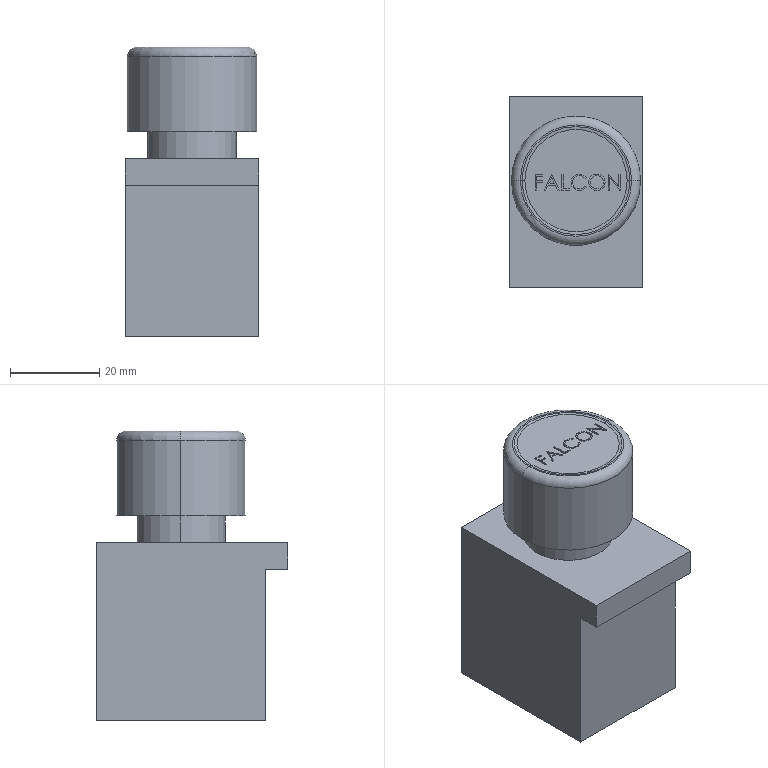Part | STEP file | Start unit | 1 solid | 83 faces | box 30 x 43 x 65 mm | volume 60814 mm3 | plane 58 | spline 17 | torus 4 | cylinder 4 | commonest cylinder face diameters 20 x2 29 x2